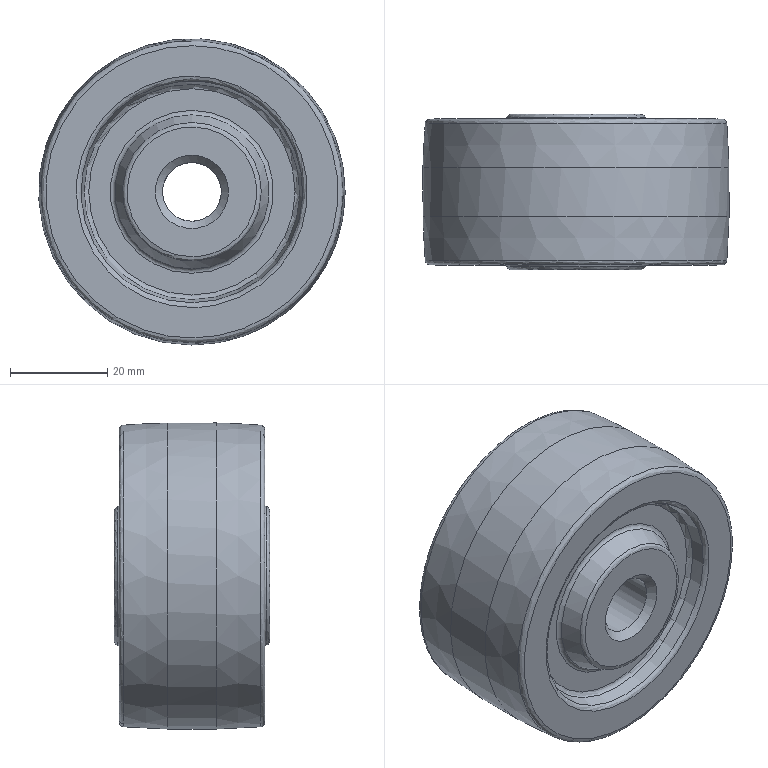Part | STEP file | 1 solid | 26 faces | box 63 x 32 x 63 mm | volume 83090 mm3 | cone 8 | plane 6 | spline 6 | torus 4 | cylinder 2 | commonest cylinder face diameters 12.1 x1 63 x1